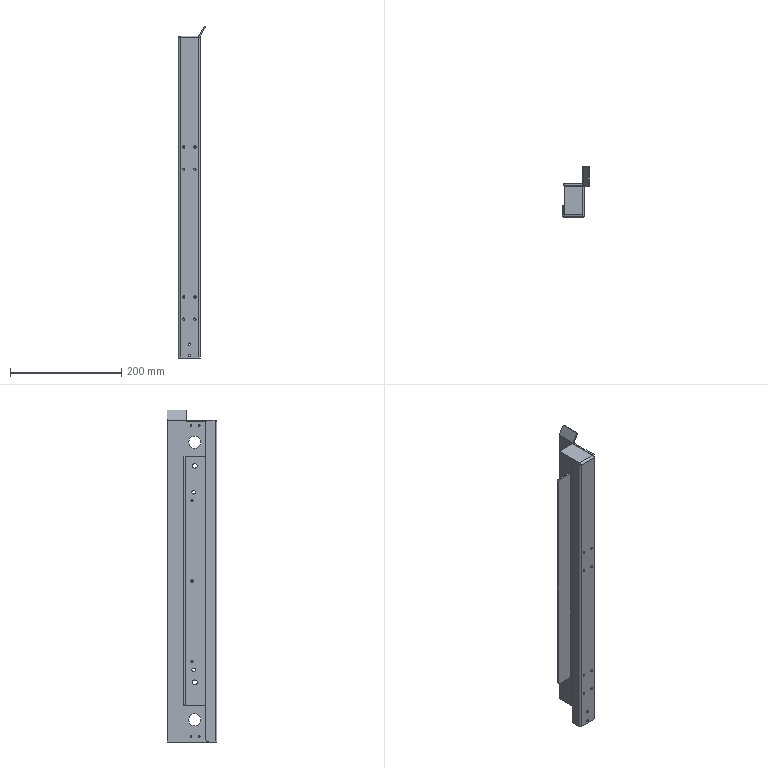Part | SolidWorks | features HoleWzd 12, EdgeFlange 6, Fillet 2, FlatPattern 2, ICE 2, SMBaseFlange 2, SheetMetal 2 | 2 solids | 122 faces | box 49.598 x 90 x 598.124 mm | volume 346794 mm3 | cylinder 74 | plane 48 | commonest cylinder face diameters 4.2 x26 3.2 x8 6.5 x8 8.6 x8 3.3 x6 0.8 x5